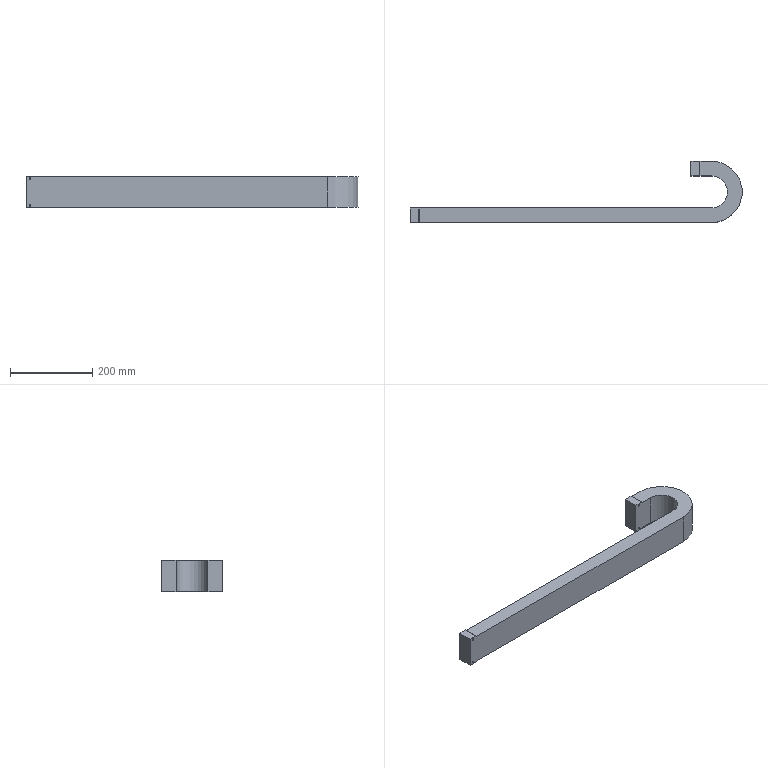Part | STEP file | Cable carrier 25x57x1000-R55-quiet-two-side-openable_cable carrier 2 | 1 solid | 26 faces | box 810 x 150 x 78 mm | volume 2572338 mm3 | plane 16 | cylinder 10 | commonest cylinder face diameters 4.2 x8 78 x1 150 x1